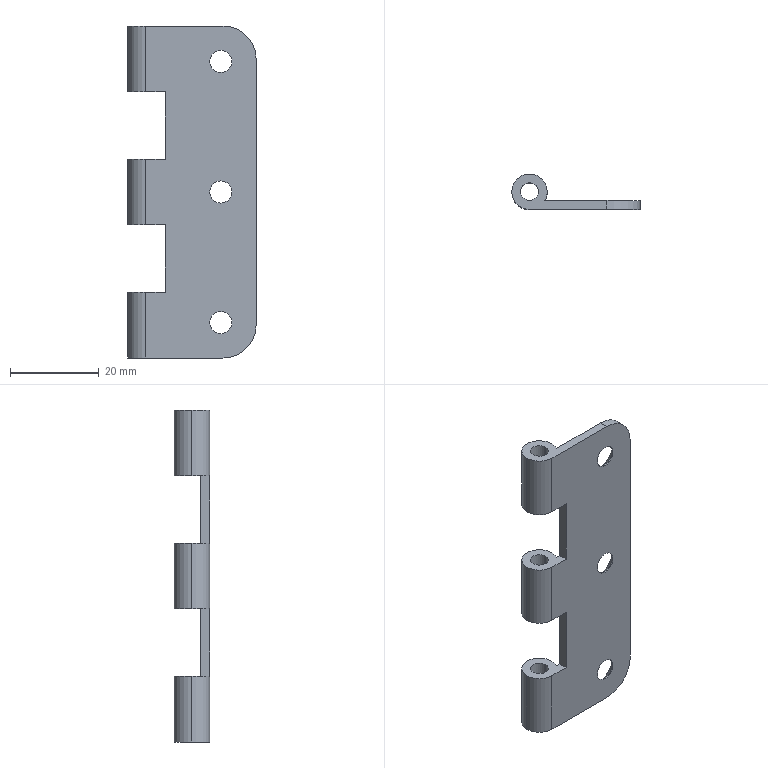Part | STEP file | 1 solid | 40 faces | box 29 x 8 x 75 mm | volume 4670 mm3 | cylinder 23 | plane 11 | cone 6 | commonest cylinder face diameters 8 x9 4 x6 5 x6 15 x2